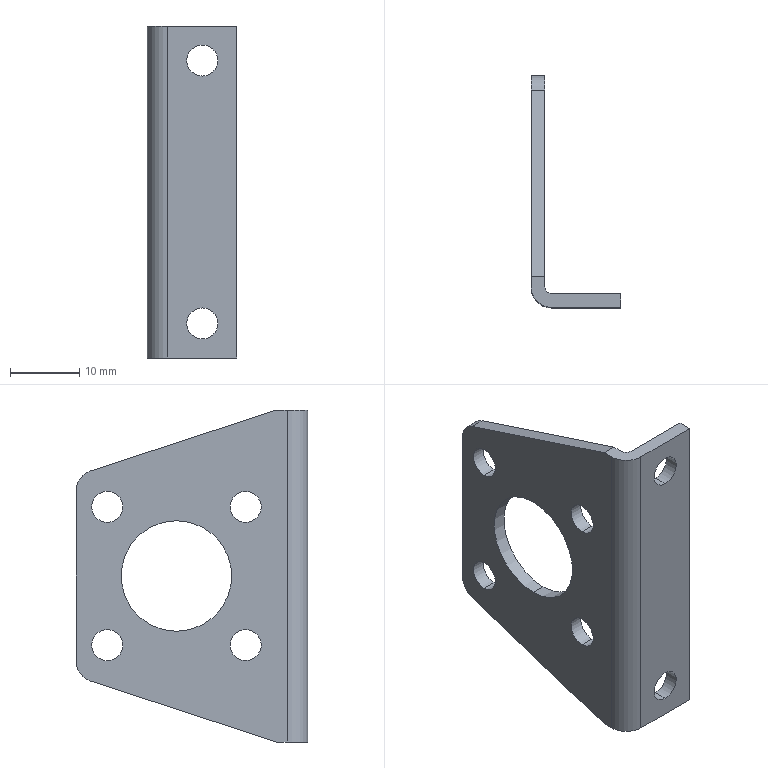Part | STEP file | _F-ACQ16LB | 1 solid | 28 faces | box 13 x 33.5 x 48 mm | volume 3042 mm3 | cylinder 18 | plane 10 | commonest cylinder face diameters 4.5 x12 6 x3 16 x2 2 x1
STEP:
#1=CARTESIAN_POINT('',(0.,19.,8.));
#2=VERTEX_POINT('',#1);
#3=CARTESIAN_POINT('',(0.,19.,-8.));
#4=VERTEX_POINT('',#3);
#5=CARTESIAN_POINT('',(0.,19.,0.));
#6=DIRECTION('',(1.,0.,0.));
#7=DIRECTION('',(0.,0.,-1.));
#8=AXIS2_PLACEMENT_3D('',#5,#6,#7);
#9=CIRCLE('',#8,8.);
#10=EDGE_CURVE('',#2,#4,#9,.T.);
#11=ORIENTED_EDGE('',*,*,#10,.F.);
#12=CARTESIAN_POINT('',(2.,19.,8.));
#13=VERTEX_POINT('',#12);
#14=CARTESIAN_POINT('',(22.,19.,8.));
#15=DIRECTION('',(1.,0.,0.));
#16=VECTOR('',#15,1000.);
#17=LINE('',#14,#16);
#18=EDGE_CURVE('',#2,#13,#17,.T.);
#19=ORIENTED_EDGE('',*,*,#18,.T.);
#20=CARTESIAN_POINT('',(2.,19.,-8.));
#21=VERTEX_POINT('',#20);
#22=CARTESIAN_POINT('',(2.,19.,0.));
#23=DIRECTION('',(1.,0.,0.));
#24=DIRECTION('',(0.,0.,-1.));
#25=AXIS2_PLACEMENT_3D('',#22,#23,#24);
#26=CIRCLE('',#25,8.);
#27=EDGE_CURVE('',#13,#21,#26,.T.);
#28=ORIENTED_EDGE('',*,*,#27,.T.);
#29=CARTESIAN_POINT('',(22.,19.,-8.));
#30=DIRECTION('',(1.,0.,0.));
#31=VECTOR('',#30,1000.);
#32=LINE('',#29,#31);
#33=EDGE_CURVE('',#4,#21,#32,.T.);
#34=ORIENTED_EDGE('',*,*,#33,.F.);
#35=EDGE_LOOP('',(#11,#19,#28,#34));
#36=FACE_OUTER_BOUND('',#35,.T.);
#37=CARTESIAN_POINT('',(22.,19.,0.));
#38=DIRECTION('',(1.,0.,0.));
#39=DIRECTION('',(0.,0.,-1.));
#40=AXIS2_PLACEMENT_3D('',#37,#38,#39);
#41=CYLINDRICAL_SURFACE('',#40,8.);
#42=ADVANCED_FACE('',(#36),#41,.F.);
#43=CARTESIAN_POINT('',(0.,9.,12.25));
#44=VERTEX_POINT('',#43);
#45=CARTESIAN_POINT('',(0.,9.,7.75));
#46=VERTEX_POINT('',#45);
#47=CARTESIAN_POINT('',(0.,9.,10.));
#48=DIRECTION('',(1.,0.,0.));
#49=DIRECTION('',(0.,0.,-1.));
#50=AXIS2_PLACEMENT_3D('',#47,#48,#49);
#51=CIRCLE('',#50,2.25);
#52=EDGE_CURVE('',#44,#46,#51,.T.);
#53=ORIENTED_EDGE('',*,*,#52,.F.);
#54=CARTESIAN_POINT('',(2.,9.,12.25));
#55=VERTEX_POINT('',#54);
#56=CARTESIAN_POINT('',(22.,9.,12.25));
#57=DIRECTION('',(1.,0.,0.));
#58=VECTOR('',#57,1000.);
#59=LINE('',#56,#58);
#60=EDGE_CURVE('',#44,#55,#59,.T.);
#61=ORIENTED_EDGE('',*,*,#60,.T.);
#62=CARTESIAN_POINT('',(2.,9.,7.75));
#63=VERTEX_POINT('',#62);
#64=CARTESIAN_POINT('',(2.,9.,10.));
#65=DIRECTION('',(1.,0.,0.));
#66=DIRECTION('',(0.,0.,-1.));
#67=AXIS2_PLACEMENT_3D('',#64,#65,#66);
#68=CIRCLE('',#67,2.25);
#69=EDGE_CURVE('',#55,#63,#68,.T.);
#70=ORIENTED_EDGE('',*,*,#69,.T.);
#71=CARTESIAN_POINT('',(22.,9.,7.75));
#72=DIRECTION('',(1.,0.,0.));
#73=VECTOR('',#72,1000.);
#74=LINE('',#71,#73);
#75=EDGE_CURVE('',#46,#63,#74,.T.);
#76=ORIENTED_EDGE('',*,*,#75,.F.);
#77=EDGE_LOOP('',(#53,#61,#70,#76));
#78=FACE_OUTER_BOUND('',#77,.T.);
#79=CARTESIAN_POINT('',(22.,9.,10.));
#80=DIRECTION('',(1.,0.,0.));
#81=DIRECTION('',(0.,0.,-1.));
#82=AXIS2_PLACEMENT_3D('',#79,#80,#81);
#83=CYLINDRICAL_SURFACE('',#82,2.25);
#84=ADVANCED_FACE('',(#78),#83,.F.);
#85=CARTESIAN_POINT('',(0.,29.,12.25));
#86=VERTEX_POINT('',#85);
#87=CARTESIAN_POINT('',(0.,29.,7.75));
#88=VERTEX_POINT('',#87);
#89=CARTESIAN_POINT('',(0.,29.,10.));
#90=DIRECTION('',(1.,0.,0.));
#91=DIRECTION('',(0.,0.,-1.));
#92=AXIS2_PLACEMENT_3D('',#89,#90,#91);
#93=CIRCLE('',#92,2.25);
#94=EDGE_CURVE('',#86,#88,#93,.T.);
#95=ORIENTED_EDGE('',*,*,#94,.F.);
#96=CARTESIAN_POINT('',(2.,29.,12.25));
#97=VERTEX_POINT('',#96);
#98=CARTESIAN_POINT('',(22.,29.,12.25));
#99=DIRECTION('',(1.,0.,0.));
#100=VECTOR('',#99,1000.);
#101=LINE('',#98,#100);
#102=EDGE_CURVE('',#86,#97,#101,.T.);
#103=ORIENTED_EDGE('',*,*,#102,.T.);
#104=CARTESIAN_POINT('',(2.,29.,7.75));
#105=VERTEX_POINT('',#104);
#106=CARTESIAN_POINT('',(2.,29.,10.));
#107=DIRECTION('',(1.,0.,0.));
#108=DIRECTION('',(0.,0.,-1.));
#109=AXIS2_PLACEMENT_3D('',#106,#107,#108);
#110=CIRCLE('',#109,2.25);
#111=EDGE_CURVE('',#97,#105,#110,.T.);
#112=ORIENTED_EDGE('',*,*,#111,.T.);
#113=CARTESIAN_POINT('',(22.,29.,7.75));
#114=DIRECTION('',(1.,0.,0.));
#115=VECTOR('',#114,1000.);
#116=LINE('',#113,#115);
#117=EDGE_CURVE('',#88,#105,#116,.T.);
#118=ORIENTED_EDGE('',*,*,#117,.F.);
#119=EDGE_LOOP('',(#95,#103,#112,#118));
#120=FACE_OUTER_BOUND('',#119,.T.);
#121=CARTESIAN_POINT('',(22.,29.,10.));
#122=DIRECTION('',(1.,0.,0.));
#123=DIRECTION('',(0.,0.,-1.));
#124=AXIS2_PLACEMENT_3D('',#121,#122,#123);
#125=CYLINDRICAL_SURFACE('',#124,2.25);
#126=ADVANCED_FACE('',(#120),#125,.F.);
#127=CARTESIAN_POINT('',(0.,29.,-7.75));
#128=VERTEX_POINT('',#127);
#129=CARTESIAN_POINT('',(0.,29.,-12.25));
#130=VERTEX_POINT('',#129);
#131=CARTESIAN_POINT('',(0.,29.,-10.));
#132=DIRECTION('',(1.,0.,0.));
#133=DIRECTION('',(0.,0.,-1.));
#134=AXIS2_PLACEMENT_3D('',#131,#132,#133);
#135=CIRCLE('',#134,2.25);
#136=EDGE_CURVE('',#128,#130,#135,.T.);
#137=ORIENTED_EDGE('',*,*,#136,.F.);
#138=CARTESIAN_POINT('',(2.,29.,-7.75));
#139=VERTEX_POINT('',#138);
#140=CARTESIAN_POINT('',(22.,29.,-7.75));
#141=DIRECTION('',(1.,0.,0.));
#142=VECTOR('',#141,1000.);
#143=LINE('',#140,#142);
#144=EDGE_CURVE('',#128,#139,#143,.T.);
#145=ORIENTED_EDGE('',*,*,#144,.T.);
#146=CARTESIAN_POINT('',(2.,29.,-12.25));
#147=VERTEX_POINT('',#146);
#148=CARTESIAN_POINT('',(2.,29.,-10.));
#149=DIRECTION('',(1.,0.,0.));
#150=DIRECTION('',(0.,0.,-1.));
#151=AXIS2_PLACEMENT_3D('',#148,#149,#150);
#152=CIRCLE('',#151,2.25);
#153=EDGE_CURVE('',#139,#147,#152,.T.);
#154=ORIENTED_EDGE('',*,*,#153,.T.);
#155=CARTESIAN_POINT('',(22.,29.,-12.25));
#156=DIRECTION('',(1.,0.,0.));
#157=VECTOR('',#156,1000.);
#158=LINE('',#155,#157);
#159=EDGE_CURVE('',#130,#147,#158,.T.);
#160=ORIENTED_EDGE('',*,*,#159,.F.);
#161=EDGE_LOOP('',(#137,#145,#154,#160));
#162=FACE_OUTER_BOUND('',#161,.T.);
#163=CARTESIAN_POINT('',(22.,29.,-10.));
#164=DIRECTION('',(1.,0.,0.));
#165=DIRECTION('',(0.,0.,-1.));
#166=AXIS2_PLACEMENT_3D('',#163,#164,#165);
#167=CYLINDRICAL_SURFACE('',#166,2.25);
#168=ADVANCED_FACE('',(#162),#167,.F.);
#169=CARTESIAN_POINT('',(0.,9.,-7.75));
#170=VERTEX_POINT('',#169);
#171=CARTESIAN_POINT('',(0.,9.,-12.25));
#172=VERTEX_POINT('',#171);
#173=CARTESIAN_POINT('',(0.,9.,-10.));
#174=DIRECTION('',(1.,0.,0.));
#175=DIRECTION('',(0.,0.,-1.));
#176=AXIS2_PLACEMENT_3D('',#173,#174,#175);
#177=CIRCLE('',#176,2.25);
#178=EDGE_CURVE('',#170,#172,#177,.T.);
#179=ORIENTED_EDGE('',*,*,#178,.F.);
#180=CARTESIAN_POINT('',(2.,9.,-7.75));
#181=VERTEX_POINT('',#180);
#182=CARTESIAN_POINT('',(22.,9.,-7.75));
#183=DIRECTION('',(1.,0.,0.));
#184=VECTOR('',#183,1000.);
#185=LINE('',#182,#184);
#186=EDGE_CURVE('',#170,#181,#185,.T.);
#187=ORIENTED_EDGE('',*,*,#186,.T.);
#188=CARTESIAN_POINT('',(2.,9.,-12.25));
#189=VERTEX_POINT('',#188);
#190=CARTESIAN_POINT('',(2.,9.,-10.));
#191=DIRECTION('',(1.,0.,0.));
#192=DIRECTION('',(0.,0.,-1.));
#193=AXIS2_PLACEMENT_3D('',#190,#191,#192);
#194=CIRCLE('',#193,2.25);
#195=EDGE_CURVE('',#181,#189,#194,.T.);
#196=ORIENTED_EDGE('',*,*,#195,.T.);
#197=CARTESIAN_POINT('',(22.,9.,-12.25));
#198=DIRECTION('',(1.,0.,0.));
#199=VECTOR('',#198,1000.);
#200=LINE('',#197,#199);
#201=EDGE_CURVE('',#172,#189,#200,.T.);
#202=ORIENTED_EDGE('',*,*,#201,.F.);
#203=EDGE_LOOP('',(#179,#187,#196,#202));
#204=FACE_OUTER_BOUND('',#203,.T.);
#205=CARTESIAN_POINT('',(22.,9.,-10.));
#206=DIRECTION('',(1.,0.,0.));
#207=DIRECTION('',(0.,0.,-1.));
#208=AXIS2_PLACEMENT_3D('',#205,#206,#207);
#209=CYLINDRICAL_SURFACE('',#208,2.25);
#210=ADVANCED_FACE('',(#204),#209,.F.);
#211=CARTESIAN_POINT('',(8.,0.,-16.75));
#212=VERTEX_POINT('',#211);
#213=CARTESIAN_POINT('',(8.,0.,-21.25));
#214=VERTEX_POINT('',#213);
#215=CARTESIAN_POINT('',(8.,0.,-19.));
#216=DIRECTION('',(0.,-1.,0.));
#217=DIRECTION('',(0.,0.,1.));
#218=AXIS2_PLACEMENT_3D('',#215,#216,#217);
#219=CIRCLE('',#218,2.25);
#220=EDGE_CURVE('',#212,#214,#219,.T.);
#221=ORIENTED_EDGE('',*,*,#220,.T.);
#222=CARTESIAN_POINT('',(8.,2.,-21.25));
#223=VERTEX_POINT('',#222);
#224=CARTESIAN_POINT('',(8.,24.,-21.25));
#225=DIRECTION('',(0.,1.,0.));
#226=VECTOR('',#225,1000.);
#227=LINE('',#224,#226);
#228=EDGE_CURVE('',#214,#223,#227,.T.);
#229=ORIENTED_EDGE('',*,*,#228,.T.);
#230=CARTESIAN_POINT('',(8.,2.,-16.75));
#231=VERTEX_POINT('',#230);
#232=CARTESIAN_POINT('',(8.,2.,-19.));
#233=DIRECTION('',(0.,1.,0.));
#234=DIRECTION('',(0.,0.,1.));
#235=AXIS2_PLACEMENT_3D('',#232,#233,#234);
#236=CIRCLE('',#235,2.25);
#237=EDGE_CURVE('',#223,#231,#236,.T.);
#238=ORIENTED_EDGE('',*,*,#237,.T.);
#239=CARTESIAN_POINT('',(8.,24.,-16.75));
#240=DIRECTION('',(0.,1.,0.));
#241=VECTOR('',#240,1000.);
#242=LINE('',#239,#241);
#243=EDGE_CURVE('',#212,#231,#242,.T.);
#244=ORIENTED_EDGE('',*,*,#243,.F.);
#245=EDGE_LOOP('',(#221,#229,#238,#244));
#246=FACE_OUTER_BOUND('',#245,.T.);
#247=CARTESIAN_POINT('',(8.,24.,-19.));
#248=DIRECTION('',(0.,1.,0.));
#249=DIRECTION('',(0.,0.,1.));
#250=AXIS2_PLACEMENT_3D('',#247,#248,#249);
#251=CYLINDRICAL_SURFACE('',#250,2.25);
#252=ADVANCED_FACE('',(#246),#251,.F.);
#253=CARTESIAN_POINT('',(8.,0.,21.25));
#254=VERTEX_POINT('',#253);
#255=CARTESIAN_POINT('',(8.,0.,16.75));
#256=VERTEX_POINT('',#255);
#257=CARTESIAN_POINT('',(8.,0.,19.));
#258=DIRECTION('',(0.,-1.,0.));
#259=DIRECTION('',(0.,0.,1.));
#260=AXIS2_PLACEMENT_3D('',#257,#258,#259);
#261=CIRCLE('',#260,2.25);
#262=EDGE_CURVE('',#254,#256,#261,.T.);
#263=ORIENTED_EDGE('',*,*,#262,.T.);
#264=CARTESIAN_POINT('',(8.,2.,16.75));
#265=VERTEX_POINT('',#264);
#266=CARTESIAN_POINT('',(8.,24.,16.75));
#267=DIRECTION('',(0.,1.,0.));
#268=VECTOR('',#267,1000.);
#269=LINE('',#266,#268);
#270=EDGE_CURVE('',#256,#265,#269,.T.);
#271=ORIENTED_EDGE('',*,*,#270,.T.);
#272=CARTESIAN_POINT('',(8.,2.,21.25));
#273=VERTEX_POINT('',#272);
#274=CARTESIAN_POINT('',(8.,2.,19.));
#275=DIRECTION('',(0.,1.,0.));
#276=DIRECTION('',(0.,0.,1.));
#277=AXIS2_PLACEMENT_3D('',#274,#275,#276);
#278=CIRCLE('',#277,2.25);
#279=EDGE_CURVE('',#265,#273,#278,.T.);
#280=ORIENTED_EDGE('',*,*,#279,.T.);
#281=CARTESIAN_POINT('',(8.,24.,21.25));
#282=DIRECTION('',(0.,1.,0.));
#283=VECTOR('',#282,1000.);
#284=LINE('',#281,#283);
#285=EDGE_CURVE('',#254,#273,#284,.T.);
#286=ORIENTED_EDGE('',*,*,#285,.F.);
#287=EDGE_LOOP('',(#263,#271,#280,#286));
#288=FACE_OUTER_BOUND('',#287,.T.);
#289=CARTESIAN_POINT('',(8.,24.,19.));
#290=DIRECTION('',(0.,1.,0.));
#291=DIRECTION('',(0.,0.,1.));
#292=AXIS2_PLACEMENT_3D('',#289,#290,#291);
#293=CYLINDRICAL_SURFACE('',#292,2.25);
#294=ADVANCED_FACE('',(#288),#293,.F.);
#295=CARTESIAN_POINT('',(2.,4.5,24.));
#296=VERTEX_POINT('',#295);
#297=CARTESIAN_POINT('',(2.,31.434,15.181));
#298=VERTEX_POINT('',#297);
#299=CARTESIAN_POINT('',(2.,4.5,24.));
#300=DIRECTION('',(0.,0.9504,-0.3112));
#301=VECTOR('',#300,1000.);
#302=LINE('',#299,#301);
#303=EDGE_CURVE('',#296,#298,#302,.T.);
#304=ORIENTED_EDGE('',*,*,#303,.F.);
#305=CARTESIAN_POINT('',(2.,3.,24.));
#306=VERTEX_POINT('',#305);
#307=CARTESIAN_POINT('',(2.,3.,24.));
#308=DIRECTION('',(0.,1.,0.));
#309=VECTOR('',#308,1000.);
#310=LINE('',#307,#309);
#311=EDGE_CURVE('',#306,#296,#310,.T.);
#312=ORIENTED_EDGE('',*,*,#311,.F.);
#313=CARTESIAN_POINT('',(2.,3.,-24.));
#314=VERTEX_POINT('',#313);
#315=CARTESIAN_POINT('',(2.,3.,24.));
#316=DIRECTION('',(0.,0.,1.));
#317=VECTOR('',#316,1000.);
#318=LINE('',#315,#317);
#319=EDGE_CURVE('',#314,#306,#318,.T.);
#320=ORIENTED_EDGE('',*,*,#319,.F.);
#321=CARTESIAN_POINT('',(2.,4.5,-24.));
#322=VERTEX_POINT('',#321);
#323=CARTESIAN_POINT('',(2.,3.,-24.));
#324=DIRECTION('',(0.,1.,0.));
#325=VECTOR('',#324,1000.);
#326=LINE('',#323,#325);
#327=EDGE_CURVE('',#314,#322,#326,.T.);
#328=ORIENTED_EDGE('',*,*,#327,.T.);
#329=CARTESIAN_POINT('',(2.,31.434,-15.181));
#330=VERTEX_POINT('',#329);
#331=CARTESIAN_POINT('',(2.,31.434,-15.181));
#332=DIRECTION('',(0.,-0.9504,-0.3112));
#333=VECTOR('',#332,1000.);
#334=LINE('',#331,#333);
#335=EDGE_CURVE('',#330,#322,#334,.T.);
#336=ORIENTED_EDGE('',*,*,#335,.F.);
#337=CARTESIAN_POINT('',(2.,33.5,-12.33));
#338=VERTEX_POINT('',#337);
#339=CARTESIAN_POINT('',(2.,30.5,-12.33));
#340=DIRECTION('',(-1.,0.,0.));
#341=DIRECTION('',(0.,0.,-1.));
#342=AXIS2_PLACEMENT_3D('',#339,#340,#341);
#343=CIRCLE('',#342,3.);
#344=EDGE_CURVE('',#338,#330,#343,.T.);
#345=ORIENTED_EDGE('',*,*,#344,.F.);
#346=CARTESIAN_POINT('',(2.,33.5,12.33));
#347=VERTEX_POINT('',#346);
#348=CARTESIAN_POINT('',(2.,33.5,24.));
#349=DIRECTION('',(0.,0.,-1.));
#350=VECTOR('',#349,1000.);
#351=LINE('',#348,#350);
#352=EDGE_CURVE('',#347,#338,#351,.T.);
#353=ORIENTED_EDGE('',*,*,#352,.F.);
#354=CARTESIAN_POINT('',(2.,30.5,12.33));
#355=DIRECTION('',(-1.,0.,0.));
#356=DIRECTION('',(0.,0.,-1.));
#357=AXIS2_PLACEMENT_3D('',#354,#355,#356);
#358=CIRCLE('',#357,3.);
#359=EDGE_CURVE('',#298,#347,#358,.T.);
#360=ORIENTED_EDGE('',*,*,#359,.F.);
#361=EDGE_LOOP('',(#304,#312,#320,#328,#336,#345,#353,#360));
#362=FACE_OUTER_BOUND('',#361,.T.);
#363=CARTESIAN_POINT('',(2.,19.,0.));
#364=DIRECTION('',(1.,0.,0.));
#365=DIRECTION('',(0.,0.,-1.));
#366=AXIS2_PLACEMENT_3D('',#363,#364,#365);
#367=CIRCLE('',#366,8.);
#368=EDGE_CURVE('',#21,#13,#367,.T.);
#369=ORIENTED_EDGE('',*,*,#368,.F.);
#370=ORIENTED_EDGE('',*,*,#27,.F.);
#371=EDGE_LOOP('',(#369,#370));
#372=FACE_BOUND('',#371,.T.);
#373=CARTESIAN_POINT('',(2.,9.,10.));
#374=DIRECTION('',(1.,0.,0.));
#375=DIRECTION('',(0.,0.,-1.));
#376=AXIS2_PLACEMENT_3D('',#373,#374,#375);
#377=CIRCLE('',#376,2.25);
#378=EDGE_CURVE('',#63,#55,#377,.T.);
#379=ORIENTED_EDGE('',*,*,#378,.F.);
#380=ORIENTED_EDGE('',*,*,#69,.F.);
#381=EDGE_LOOP('',(#379,#380));
#382=FACE_BOUND('',#381,.T.);
#383=CARTESIAN_POINT('',(2.,29.,10.));
#384=DIRECTION('',(1.,0.,0.));
#385=DIRECTION('',(0.,0.,-1.));
#386=AXIS2_PLACEMENT_3D('',#383,#384,#385);
#387=CIRCLE('',#386,2.25);
#388=EDGE_CURVE('',#105,#97,#387,.T.);
#389=ORIENTED_EDGE('',*,*,#388,.F.);
#390=ORIENTED_EDGE('',*,*,#111,.F.);
#391=EDGE_LOOP('',(#389,#390));
#392=FACE_BOUND('',#391,.T.);
#393=CARTESIAN_POINT('',(2.,29.,-10.));
#394=DIRECTION('',(1.,0.,0.));
#395=DIRECTION('',(0.,0.,-1.));
#396=AXIS2_PLACEMENT_3D('',#393,#394,#395);
#397=CIRCLE('',#396,2.25);
#398=EDGE_CURVE('',#147,#139,#397,.T.);
#399=ORIENTED_EDGE('',*,*,#398,.F.);
#400=ORIENTED_EDGE('',*,*,#153,.F.);
#401=EDGE_LOOP('',(#399,#400));
#402=FACE_BOUND('',#401,.T.);
#403=CARTESIAN_POINT('',(2.,9.,-10.));
#404=DIRECTION('',(1.,0.,0.));
#405=DIRECTION('',(0.,0.,-1.));
#406=AXIS2_PLACEMENT_3D('',#403,#404,#405);
#407=CIRCLE('',#406,2.25);
#408=EDGE_CURVE('',#189,#181,#407,.T.);
#409=ORIENTED_EDGE('',*,*,#408,.F.);
#410=ORIENTED_EDGE('',*,*,#195,.F.);
#411=EDGE_LOOP('',(#409,#410));
#412=FACE_BOUND('',#411,.T.);
#413=CARTESIAN_POINT('',(2.,3.,24.));
#414=DIRECTION('',(-1.,0.,0.));
#415=DIRECTION('',(0.,0.,1.));
#416=AXIS2_PLACEMENT_3D('',#413,#414,#415);
#417=PLANE('',#416);
#418=ADVANCED_FACE('',(#362,#372,#382,#392,#402,#412),#417,.F.);
#419=CARTESIAN_POINT('',(0.,33.5,12.33));
#420=VERTEX_POINT('',#419);
#421=CARTESIAN_POINT('',(22.,33.5,12.33));
#422=DIRECTION('',(-1.,0.,0.));
#423=VECTOR('',#422,1000.);
#424=LINE('',#421,#423);
#425=EDGE_CURVE('',#347,#420,#424,.T.);
#426=ORIENTED_EDGE('',*,*,#425,.T.);
#427=CARTESIAN_POINT('',(0.,31.434,15.181));
#428=VERTEX_POINT('',#427);
#429=CARTESIAN_POINT('',(0.,30.5,12.33));
#430=DIRECTION('',(1.,0.,0.));
#431=DIRECTION('',(0.,0.,-1.));
#432=AXIS2_PLACEMENT_3D('',#429,#430,#431);
#433=CIRCLE('',#432,3.);
#434=EDGE_CURVE('',#420,#428,#433,.T.);
#435=ORIENTED_EDGE('',*,*,#434,.T.);
#436=CARTESIAN_POINT('',(22.,31.434,15.181));
#437=DIRECTION('',(1.,0.,0.));
#438=VECTOR('',#437,1000.);
#439=LINE('',#436,#438);
#440=EDGE_CURVE('',#428,#298,#439,.T.);
#441=ORIENTED_EDGE('',*,*,#440,.T.);
#442=ORIENTED_EDGE('',*,*,#359,.T.);
#443=EDGE_LOOP('',(#426,#435,#441,#442));
#444=FACE_OUTER_BOUND('',#443,.T.);
#445=CARTESIAN_POINT('',(22.,30.5,12.33));
#446=DIRECTION('',(1.,0.,0.));
#447=DIRECTION('',(0.,0.,-1.));
#448=AXIS2_PLACEMENT_3D('',#445,#446,#447);
#449=CYLINDRICAL_SURFACE('',#448,3.);
#450=ADVANCED_FACE('',(#444),#449,.T.);
#451=ORIENTED_EDGE('',*,*,#303,.T.);
#452=ORIENTED_EDGE('',*,*,#440,.F.);
#453=CARTESIAN_POINT('',(0.,4.5,24.));
#454=VERTEX_POINT('',#453);
#455=CARTESIAN_POINT('',(0.,31.434,15.181));
#456=DIRECTION('',(0.,0.9504,-0.3112));
#457=VECTOR('',#456,1000.);
#458=LINE('',#455,#457);
#459=EDGE_CURVE('',#454,#428,#458,.T.);
#460=ORIENTED_EDGE('',*,*,#459,.F.);
#461=CARTESIAN_POINT('',(22.,4.5,24.));
#462=DIRECTION('',(-1.,0.,0.));
#463=VECTOR('',#462,1000.);
#464=LINE('',#461,#463);
#465=EDGE_CURVE('',#296,#454,#464,.T.);
#466=ORIENTED_EDGE('',*,*,#465,.F.);
#467=EDGE_LOOP('',(#451,#452,#460,#466));
#468=FACE_OUTER_BOUND('',#467,.T.);
#469=CARTESIAN_POINT('',(22.,31.434,15.181));
#470=DIRECTION('',(0.,-0.3112,-0.9504));
#471=DIRECTION('',(0.,0.9504,-0.3112));
#472=AXIS2_PLACEMENT_3D('',#469,#470,#471);
#473=PLANE('',#472);
#474=ADVANCED_FACE('',(#468),#473,.F.);
#475=ORIENTED_EDGE('',*,*,#319,.T.);
#476=CARTESIAN_POINT('',(3.,2.,24.));
#477=VERTEX_POINT('',#476);
#478=CARTESIAN_POINT('',(3.,3.,24.));
#479=DIRECTION('',(0.,0.,-1.));
#480=DIRECTION('',(1.,0.,0.));
#481=AXIS2_PLACEMENT_3D('',#478,#479,#480);
#482=CIRCLE('',#481,1.);
#483=EDGE_CURVE('',#477,#306,#482,.T.);
#484=ORIENTED_EDGE('',*,*,#483,.F.);
#485=CARTESIAN_POINT('',(3.,2.,-24.));
#486=VERTEX_POINT('',#485);
#487=CARTESIAN_POINT('',(3.,2.,24.));
#488=DIRECTION('',(0.,0.,1.));
#489=VECTOR('',#488,1000.);
#490=LINE('',#487,#489);
#491=EDGE_CURVE('',#486,#477,#490,.T.);
#492=ORIENTED_EDGE('',*,*,#491,.F.);
#493=CARTESIAN_POINT('',(3.,3.,-24.));
#494=DIRECTION('',(0.,0.,-1.));
#495=DIRECTION('',(1.,0.,0.));
#496=AXIS2_PLACEMENT_3D('',#493,#494,#495);
#497=CIRCLE('',#496,1.);
#498=EDGE_CURVE('',#486,#314,#497,.T.);
#499=ORIENTED_EDGE('',*,*,#498,.T.);
#500=EDGE_LOOP('',(#475,#484,#492,#499));
#501=FACE_OUTER_BOUND('',#500,.T.);
#502=CARTESIAN_POINT('',(3.,3.,24.));
#503=DIRECTION('',(0.,0.,1.));
#504=DIRECTION('',(1.,0.,0.));
#505=AXIS2_PLACEMENT_3D('',#502,#503,#504);
#506=CYLINDRICAL_SURFACE('',#505,1.);
#507=ADVANCED_FACE('',(#501),#506,.F.);
#508=ORIENTED_EDGE('',*,*,#335,.T.);
#509=CARTESIAN_POINT('',(0.,4.5,-24.));
#510=VERTEX_POINT('',#509);
#511=CARTESIAN_POINT('',(22.,4.5,-24.));
#512=DIRECTION('',(1.,0.,0.));
#513=VECTOR('',#512,1000.);
#514=LINE('',#511,#513);
#515=EDGE_CURVE('',#510,#322,#514,.T.);
#516=ORIENTED_EDGE('',*,*,#515,.F.);
#517=CARTESIAN_POINT('',(0.,31.434,-15.181));
#518=VERTEX_POINT('',#517);
#519=CARTESIAN_POINT('',(0.,4.5,-24.));
#520=DIRECTION('',(0.,-0.9504,-0.3112));
#521=VECTOR('',#520,1000.);
#522=LINE('',#519,#521);
#523=EDGE_CURVE('',#518,#510,#522,.T.);
#524=ORIENTED_EDGE('',*,*,#523,.F.);
#525=CARTESIAN_POINT('',(22.,31.434,-15.181));
#526=DIRECTION('',(-1.,0.,0.));
#527=VECTOR('',#526,1000.);
#528=LINE('',#525,#527);
#529=EDGE_CURVE('',#330,#518,#528,.T.);
#530=ORIENTED_EDGE('',*,*,#529,.F.);
#531=EDGE_LOOP('',(#508,#516,#524,#530));
#532=FACE_OUTER_BOUND('',#531,.T.);
#533=CARTESIAN_POINT('',(22.,4.5,-24.));
#534=DIRECTION('',(0.,-0.3112,0.9504));
#535=DIRECTION('',(0.,-0.9504,-0.3112));
#536=AXIS2_PLACEMENT_3D('',#533,#534,#535);
#537=PLANE('',#536);
#538=ADVANCED_FACE('',(#532),#537,.F.);
#539=ORIENTED_EDGE('',*,*,#529,.T.);
#540=CARTESIAN_POINT('',(0.,33.5,-12.33));
#541=VERTEX_POINT('',#540);
#542=CARTESIAN_POINT('',(0.,30.5,-12.33));
#543=DIRECTION('',(1.,0.,0.));
#544=DIRECTION('',(0.,0.,-1.));
#545=AXIS2_PLACEMENT_3D('',#542,#543,#544);
#546=CIRCLE('',#545,3.);
#547=EDGE_CURVE('',#518,#541,#546,.T.);
#548=ORIENTED_EDGE('',*,*,#547,.T.);
#549=CARTESIAN_POINT('',(22.,33.5,-12.33));
#550=DIRECTION('',(1.,0.,0.));
#551=VECTOR('',#550,1000.);
#552=LINE('',#549,#551);
#553=EDGE_CURVE('',#541,#338,#552,.T.);
#554=ORIENTED_EDGE('',*,*,#553,.T.);
#555=ORIENTED_EDGE('',*,*,#344,.T.);
#556=EDGE_LOOP('',(#539,#548,#554,#555));
#557=FACE_OUTER_BOUND('',#556,.T.);
#558=CARTESIAN_POINT('',(22.,30.5,-12.33));
#559=DIRECTION('',(1.,0.,0.));
#560=DIRECTION('',(0.,0.,-1.));
#561=AXIS2_PLACEMENT_3D('',#558,#559,#560);
#562=CYLINDRICAL_SURFACE('',#561,3.);
#563=ADVANCED_FACE('',(#557),#562,.T.);
#564=ORIENTED_EDGE('',*,*,#425,.F.);
#565=ORIENTED_EDGE('',*,*,#352,.T.);
#566=ORIENTED_EDGE('',*,*,#553,.F.);
#567=CARTESIAN_POINT('',(0.,33.5,24.));
#568=DIRECTION('',(0.,0.,-1.));
#569=VECTOR('',#568,1000.);
#570=LINE('',#567,#569);
#571=EDGE_CURVE('',#420,#541,#570,.T.);
#572=ORIENTED_EDGE('',*,*,#571,.F.);
#573=EDGE_LOOP('',(#564,#565,#566,#572));
#574=FACE_OUTER_BOUND('',#573,.T.);
#575=CARTESIAN_POINT('',(2.,33.5,24.));
#576=DIRECTION('',(0.,-1.,0.));
#577=DIRECTION('',(0.,0.,-1.));
#578=AXIS2_PLACEMENT_3D('',#575,#576,#577);
#579=PLANE('',#578);
#580=ADVANCED_FACE('',(#574),#579,.F.);
#581=ORIENTED_EDGE('',*,*,#18,.F.);
#582=CARTESIAN_POINT('',(0.,19.,0.));
#583=DIRECTION('',(1.,0.,0.));
#584=DIRECTION('',(0.,0.,-1.));
#585=AXIS2_PLACEMENT_3D('',#582,#583,#584);
#586=CIRCLE('',#585,8.);
#587=EDGE_CURVE('',#4,#2,#586,.T.);
#588=ORIENTED_EDGE('',*,*,#587,.F.);
#589=ORIENTED_EDGE('',*,*,#33,.T.);
#590=ORIENTED_EDGE('',*,*,#368,.T.);
#591=EDGE_LOOP('',(#581,#588,#589,#590));
#592=FACE_OUTER_BOUND('',#591,.T.);
#593=CARTESIAN_POINT('',(22.,19.,0.));
#594=DIRECTION('',(1.,0.,0.));
#595=DIRECTION('',(0.,0.,-1.));
#596=AXIS2_PLACEMENT_3D('',#593,#594,#595);
#597=CYLINDRICAL_SURFACE('',#596,8.);
#598=ADVANCED_FACE('',(#592),#597,.F.);
#599=ORIENTED_EDGE('',*,*,#60,.F.);
#600=CARTESIAN_POINT('',(0.,9.,10.));
#601=DIRECTION('',(1.,0.,0.));
#602=DIRECTION('',(0.,0.,-1.));
#603=AXIS2_PLACEMENT_3D('',#600,#601,#602);
#604=CIRCLE('',#603,2.25);
#605=EDGE_CURVE('',#46,#44,#604,.T.);
#606=ORIENTED_EDGE('',*,*,#605,.F.);
#607=ORIENTED_EDGE('',*,*,#75,.T.);
#608=ORIENTED_EDGE('',*,*,#378,.T.);
#609=EDGE_LOOP('',(#599,#606,#607,#608));
#610=FACE_OUTER_BOUND('',#609,.T.);
#611=CARTESIAN_POINT('',(22.,9.,10.));
#612=DIRECTION('',(1.,0.,0.));
#613=DIRECTION('',(0.,0.,-1.));
#614=AXIS2_PLACEMENT_3D('',#611,#612,#613);
#615=CYLINDRICAL_SURFACE('',#614,2.25);
#616=ADVANCED_FACE('',(#610),#615,.F.);
#617=ORIENTED_EDGE('',*,*,#102,.F.);
#618=CARTESIAN_POINT('',(0.,29.,10.));
#619=DIRECTION('',(1.,0.,0.));
#620=DIRECTION('',(0.,0.,-1.));
#621=AXIS2_PLACEMENT_3D('',#618,#619,#620);
#622=CIRCLE('',#621,2.25);
#623=EDGE_CURVE('',#88,#86,#622,.T.);
#624=ORIENTED_EDGE('',*,*,#623,.F.);
#625=ORIENTED_EDGE('',*,*,#117,.T.);
#626=ORIENTED_EDGE('',*,*,#388,.T.);
#627=EDGE_LOOP('',(#617,#624,#625,#626));
#628=FACE_OUTER_BOUND('',#627,.T.);
#629=CARTESIAN_POINT('',(22.,29.,10.));
#630=DIRECTION('',(1.,0.,0.));
#631=DIRECTION('',(0.,0.,-1.));
#632=AXIS2_PLACEMENT_3D('',#629,#630,#631);
#633=CYLINDRICAL_SURFACE('',#632,2.25);
#634=ADVANCED_FACE('',(#628),#633,.F.);
#635=ORIENTED_EDGE('',*,*,#144,.F.);
#636=CARTESIAN_POINT('',(0.,29.,-10.));
#637=DIRECTION('',(1.,0.,0.));
#638=DIRECTION('',(0.,0.,-1.));
#639=AXIS2_PLACEMENT_3D('',#636,#637,#638);
#640=CIRCLE('',#639,2.25);
#641=EDGE_CURVE('',#130,#128,#640,.T.);
#642=ORIENTED_EDGE('',*,*,#641,.F.);
#643=ORIENTED_EDGE('',*,*,#159,.T.);
#644=ORIENTED_EDGE('',*,*,#398,.T.);
#645=EDGE_LOOP('',(#635,#642,#643,#644));
#646=FACE_OUTER_BOUND('',#645,.T.);
#647=CARTESIAN_POINT('',(22.,29.,-10.));
#648=DIRECTION('',(1.,0.,0.));
#649=DIRECTION('',(0.,0.,-1.));
#650=AXIS2_PLACEMENT_3D('',#647,#648,#649);
#651=CYLINDRICAL_SURFACE('',#650,2.25);
#652=ADVANCED_FACE('',(#646),#651,.F.);
#653=ORIENTED_EDGE('',*,*,#186,.F.);
#654=CARTESIAN_POINT('',(0.,9.,-10.));
#655=DIRECTION('',(1.,0.,0.));
#656=DIRECTION('',(0.,0.,-1.));
#657=AXIS2_PLACEMENT_3D('',#654,#655,#656);
#658=CIRCLE('',#657,2.25);
#659=EDGE_CURVE('',#172,#170,#658,.T.);
#660=ORIENTED_EDGE('',*,*,#659,.F.);
#661=ORIENTED_EDGE('',*,*,#201,.T.);
#662=ORIENTED_EDGE('',*,*,#408,.T.);
#663=EDGE_LOOP('',(#653,#660,#661,#662));
#664=FACE_OUTER_BOUND('',#663,.T.);
#665=CARTESIAN_POINT('',(22.,9.,-10.));
#666=DIRECTION('',(1.,0.,0.));
#667=DIRECTION('',(0.,0.,-1.));
#668=AXIS2_PLACEMENT_3D('',#665,#666,#667);
#669=CYLINDRICAL_SURFACE('',#668,2.25);
#670=ADVANCED_FACE('',(#664),#669,.F.);
#671=ORIENTED_EDGE('',*,*,#459,.T.);
#672=ORIENTED_EDGE('',*,*,#434,.F.);
#673=ORIENTED_EDGE('',*,*,#571,.T.);
#674=ORIENTED_EDGE('',*,*,#547,.F.);
#675=ORIENTED_EDGE('',*,*,#523,.T.);
#676=CARTESIAN_POINT('',(0.,3.,-24.));
#677=VERTEX_POINT('',#676);
#678=CARTESIAN_POINT('',(0.,33.5,-24.));
#679=DIRECTION('',(0.,1.,0.));
#680=VECTOR('',#679,1000.);
#681=LINE('',#678,#680);
#682=EDGE_CURVE('',#677,#510,#681,.T.);
#683=ORIENTED_EDGE('',*,*,#682,.F.);
#684=CARTESIAN_POINT('',(0.,3.,24.));
#685=VERTEX_POINT('',#684);
#686=CARTESIAN_POINT('',(0.,3.,24.));
#687=DIRECTION('',(0.,0.,-1.));
#688=VECTOR('',#687,1000.);
#689=LINE('',#686,#688);
#690=EDGE_CURVE('',#685,#677,#689,.T.);
#691=ORIENTED_EDGE('',*,*,#690,.F.);
#692=CARTESIAN_POINT('',(0.,33.5,24.));
#693=DIRECTION('',(0.,-1.,0.));
#694=VECTOR('',#693,1000.);
#695=LINE('',#692,#694);
#696=EDGE_CURVE('',#454,#685,#695,.T.);
#697=ORIENTED_EDGE('',*,*,#696,.F.);
#698=EDGE_LOOP('',(#671,#672,#673,#674,#675,#683,#691,#697));
#699=FACE_OUTER_BOUND('',#698,.T.);
#700=ORIENTED_EDGE('',*,*,#587,.T.);
#701=ORIENTED_EDGE('',*,*,#10,.T.);
#702=EDGE_LOOP('',(#700,#701));
#703=FACE_BOUND('',#702,.T.);
#704=ORIENTED_EDGE('',*,*,#605,.T.);
#705=ORIENTED_EDGE('',*,*,#52,.T.);
#706=EDGE_LOOP('',(#704,#705));
#707=FACE_BOUND('',#706,.T.);
#708=ORIENTED_EDGE('',*,*,#623,.T.);
#709=ORIENTED_EDGE('',*,*,#94,.T.);
#710=EDGE_LOOP('',(#708,#709));
#711=FACE_BOUND('',#710,.T.);
#712=ORIENTED_EDGE('',*,*,#641,.T.);
#713=ORIENTED_EDGE('',*,*,#136,.T.);
#714=EDGE_LOOP('',(#712,#713));
#715=FACE_BOUND('',#714,.T.);
#716=ORIENTED_EDGE('',*,*,#659,.T.);
#717=ORIENTED_EDGE('',*,*,#178,.T.);
#718=EDGE_LOOP('',(#716,#717));
#719=FACE_BOUND('',#718,.T.);
#720=CARTESIAN_POINT('',(0.,33.5,24.));
#721=DIRECTION('',(1.,0.,0.));
#722=DIRECTION('',(0.,0.,-1.));
#723=AXIS2_PLACEMENT_3D('',#720,#721,#722);
#724=PLANE('',#723);
#725=ADVANCED_FACE('',(#699,#703,#707,#711,#715,#719),#724,.F.);
#726=ORIENTED_EDGE('',*,*,#483,.T.);
#727=ORIENTED_EDGE('',*,*,#311,.T.);
#728=ORIENTED_EDGE('',*,*,#465,.T.);
#729=ORIENTED_EDGE('',*,*,#696,.T.);
#730=CARTESIAN_POINT('',(3.,0.,24.));
#731=VERTEX_POINT('',#730);
#732=CARTESIAN_POINT('',(3.,3.,24.));
#733=DIRECTION('',(0.,0.,1.));
#734=DIRECTION('',(1.,0.,0.));
#735=AXIS2_PLACEMENT_3D('',#732,#733,#734);
#736=CIRCLE('',#735,3.);
#737=EDGE_CURVE('',#685,#731,#736,.T.);
#738=ORIENTED_EDGE('',*,*,#737,.T.);
#739=CARTESIAN_POINT('',(13.,0.,24.));
#740=VERTEX_POINT('',#739);
#741=CARTESIAN_POINT('',(3.,0.,24.));
#742=DIRECTION('',(1.,0.,0.));
#743=VECTOR('',#742,1000.);
#744=LINE('',#741,#743);
#745=EDGE_CURVE('',#731,#740,#744,.T.);
#746=ORIENTED_EDGE('',*,*,#745,.T.);
#747=CARTESIAN_POINT('',(13.,2.,24.));
#748=VERTEX_POINT('',#747);
#749=CARTESIAN_POINT('',(13.,3.,24.));
#750=DIRECTION('',(0.,1.,0.));
#751=VECTOR('',#750,1000.);
#752=LINE('',#749,#751);
#753=EDGE_CURVE('',#740,#748,#752,.T.);
#754=ORIENTED_EDGE('',*,*,#753,.T.);
#755=CARTESIAN_POINT('',(3.,2.,24.));
#756=DIRECTION('',(-1.,0.,0.));
#757=VECTOR('',#756,1000.);
#758=LINE('',#755,#757);
#759=EDGE_CURVE('',#748,#477,#758,.T.);
#760=ORIENTED_EDGE('',*,*,#759,.T.);
#761=EDGE_LOOP('',(#726,#727,#728,#729,#738,#746,#754,#760));
#762=FACE_OUTER_BOUND('',#761,.T.);
#763=CARTESIAN_POINT('',(3.,3.,24.));
#764=DIRECTION('',(0.,0.,1.));
#765=DIRECTION('',(1.,0.,0.));
#766=AXIS2_PLACEMENT_3D('',#763,#764,#765);
#767=PLANE('',#766);
#768=ADVANCED_FACE('',(#762),#767,.T.);
#769=ORIENTED_EDGE('',*,*,#491,.T.);
#770=ORIENTED_EDGE('',*,*,#759,.F.);
#771=CARTESIAN_POINT('',(13.,2.,-24.));
#772=VERTEX_POINT('',#771);
#773=CARTESIAN_POINT('',(13.,2.,24.));
#774=DIRECTION('',(0.,0.,1.));
#775=VECTOR('',#774,1000.);
#776=LINE('',#773,#775);
#777=EDGE_CURVE('',#772,#748,#776,.T.);
#778=ORIENTED_EDGE('',*,*,#777,.F.);
#779=CARTESIAN_POINT('',(13.,2.,-24.));
#780=DIRECTION('',(1.,0.,0.));
#781=VECTOR('',#780,1000.);
#782=LINE('',#779,#781);
#783=EDGE_CURVE('',#486,#772,#782,.T.);
#784=ORIENTED_EDGE('',*,*,#783,.F.);
#785=EDGE_LOOP('',(#769,#770,#778,#784));
#786=FACE_OUTER_BOUND('',#785,.T.);
#787=CARTESIAN_POINT('',(8.,2.,-19.));
#788=DIRECTION('',(0.,1.,0.));
#789=DIRECTION('',(0.,0.,1.));
#790=AXIS2_PLACEMENT_3D('',#787,#788,#789);
#791=CIRCLE('',#790,2.25);
#792=EDGE_CURVE('',#231,#223,#791,.T.);
#793=ORIENTED_EDGE('',*,*,#792,.F.);
#794=ORIENTED_EDGE('',*,*,#237,.F.);
#795=EDGE_LOOP('',(#793,#794));
#796=FACE_BOUND('',#795,.T.);
#797=CARTESIAN_POINT('',(8.,2.,19.));
#798=DIRECTION('',(0.,1.,0.));
#799=DIRECTION('',(0.,0.,1.));
#800=AXIS2_PLACEMENT_3D('',#797,#798,#799);
#801=CIRCLE('',#800,2.25);
#802=EDGE_CURVE('',#273,#265,#801,.T.);
#803=ORIENTED_EDGE('',*,*,#802,.F.);
#804=ORIENTED_EDGE('',*,*,#279,.F.);
#805=EDGE_LOOP('',(#803,#804));
#806=FACE_BOUND('',#805,.T.);
#807=CARTESIAN_POINT('',(13.,2.,24.));
#808=DIRECTION('',(0.,-1.,0.));
#809=DIRECTION('',(0.,0.,-1.));
#810=AXIS2_PLACEMENT_3D('',#807,#808,#809);
#811=PLANE('',#810);
#812=ADVANCED_FACE('',(#786,#796,#806),#811,.F.);
#813=ORIENTED_EDGE('',*,*,#515,.T.);
#814=ORIENTED_EDGE('',*,*,#327,.F.);
#815=ORIENTED_EDGE('',*,*,#498,.F.);
#816=ORIENTED_EDGE('',*,*,#783,.T.);
#817=CARTESIAN_POINT('',(13.,0.,-24.));
#818=VERTEX_POINT('',#817);
#819=CARTESIAN_POINT('',(13.,3.,-24.));
#820=DIRECTION('',(0.,1.,0.));
#821=VECTOR('',#820,1000.);
#822=LINE('',#819,#821);
#823=EDGE_CURVE('',#818,#772,#822,.T.);
#824=ORIENTED_EDGE('',*,*,#823,.F.);
#825=CARTESIAN_POINT('',(3.,0.,-24.));
#826=VERTEX_POINT('',#825);
#827=CARTESIAN_POINT('',(3.,0.,-24.));
#828=DIRECTION('',(1.,0.,0.));
#829=VECTOR('',#828,1000.);
#830=LINE('',#827,#829);
#831=EDGE_CURVE('',#826,#818,#830,.T.);
#832=ORIENTED_EDGE('',*,*,#831,.F.);
#833=CARTESIAN_POINT('',(3.,3.,-24.));
#834=DIRECTION('',(0.,0.,1.));
#835=DIRECTION('',(1.,0.,0.));
#836=AXIS2_PLACEMENT_3D('',#833,#834,#835);
#837=CIRCLE('',#836,3.);
#838=EDGE_CURVE('',#677,#826,#837,.T.);
#839=ORIENTED_EDGE('',*,*,#838,.F.);
#840=ORIENTED_EDGE('',*,*,#682,.T.);
#841=EDGE_LOOP('',(#813,#814,#815,#816,#824,#832,#839,#840));
#842=FACE_OUTER_BOUND('',#841,.T.);
#843=CARTESIAN_POINT('',(3.,3.,-24.));
#844=DIRECTION('',(0.,0.,1.));
#845=DIRECTION('',(1.,0.,0.));
#846=AXIS2_PLACEMENT_3D('',#843,#844,#845);
#847=PLANE('',#846);
#848=ADVANCED_FACE('',(#842),#847,.F.);
#849=ORIENTED_EDGE('',*,*,#737,.F.);
#850=ORIENTED_EDGE('',*,*,#690,.T.);
#851=ORIENTED_EDGE('',*,*,#838,.T.);
#852=CARTESIAN_POINT('',(3.,0.,24.));
#853=DIRECTION('',(0.,0.,1.));
#854=VECTOR('',#853,1000.);
#855=LINE('',#852,#854);
#856=EDGE_CURVE('',#826,#731,#855,.T.);
#857=ORIENTED_EDGE('',*,*,#856,.T.);
#858=EDGE_LOOP('',(#849,#850,#851,#857));
#859=FACE_OUTER_BOUND('',#858,.T.);
#860=CARTESIAN_POINT('',(3.,3.,24.));
#861=DIRECTION('',(0.,0.,1.));
#862=DIRECTION('',(1.,0.,0.));
#863=AXIS2_PLACEMENT_3D('',#860,#861,#862);
#864=CYLINDRICAL_SURFACE('',#863,3.);
#865=ADVANCED_FACE('',(#859),#864,.T.);
#866=ORIENTED_EDGE('',*,*,#777,.T.);
#867=ORIENTED_EDGE('',*,*,#753,.F.);
#868=CARTESIAN_POINT('',(13.,0.,24.));
#869=DIRECTION('',(0.,0.,1.));
#870=VECTOR('',#869,1000.);
#871=LINE('',#868,#870);
#872=EDGE_CURVE('',#818,#740,#871,.T.);
#873=ORIENTED_EDGE('',*,*,#872,.F.);
#874=ORIENTED_EDGE('',*,*,#823,.T.);
#875=EDGE_LOOP('',(#866,#867,#873,#874));
#876=FACE_OUTER_BOUND('',#875,.T.);
#877=CARTESIAN_POINT('',(13.,0.,24.));
#878=DIRECTION('',(-1.,0.,0.));
#879=DIRECTION('',(0.,0.,1.));
#880=AXIS2_PLACEMENT_3D('',#877,#878,#879);
#881=PLANE('',#880);
#882=ADVANCED_FACE('',(#876),#881,.F.);
#883=ORIENTED_EDGE('',*,*,#872,.T.);
#884=ORIENTED_EDGE('',*,*,#745,.F.);
#885=ORIENTED_EDGE('',*,*,#856,.F.);
#886=ORIENTED_EDGE('',*,*,#831,.T.);
#887=EDGE_LOOP('',(#883,#884,#885,#886));
#888=FACE_OUTER_BOUND('',#887,.T.);
#889=ORIENTED_EDGE('',*,*,#220,.F.);
#890=CARTESIAN_POINT('',(8.,0.,-19.));
#891=DIRECTION('',(0.,-1.,0.));
#892=DIRECTION('',(0.,0.,1.));
#893=AXIS2_PLACEMENT_3D('',#890,#891,#892);
#894=CIRCLE('',#893,2.25);
#895=EDGE_CURVE('',#214,#212,#894,.T.);
#896=ORIENTED_EDGE('',*,*,#895,.F.);
#897=EDGE_LOOP('',(#889,#896));
#898=FACE_BOUND('',#897,.T.);
#899=ORIENTED_EDGE('',*,*,#262,.F.);
#900=CARTESIAN_POINT('',(8.,0.,19.));
#901=DIRECTION('',(0.,-1.,0.));
#902=DIRECTION('',(0.,0.,1.));
#903=AXIS2_PLACEMENT_3D('',#900,#901,#902);
#904=CIRCLE('',#903,2.25);
#905=EDGE_CURVE('',#256,#254,#904,.T.);
#906=ORIENTED_EDGE('',*,*,#905,.F.);
#907=EDGE_LOOP('',(#899,#906));
#908=FACE_BOUND('',#907,.T.);
#909=CARTESIAN_POINT('',(3.,0.,24.));
#910=DIRECTION('',(0.,1.,0.));
#911=DIRECTION('',(0.,0.,1.));
#912=AXIS2_PLACEMENT_3D('',#909,#910,#911);
#913=PLANE('',#912);
#914=ADVANCED_FACE('',(#888,#898,#908),#913,.F.);
#915=ORIENTED_EDGE('',*,*,#228,.F.);
#916=ORIENTED_EDGE('',*,*,#895,.T.);
#917=ORIENTED_EDGE('',*,*,#243,.T.);
#918=ORIENTED_EDGE('',*,*,#792,.T.);
#919=EDGE_LOOP('',(#915,#916,#917,#918));
#920=FACE_OUTER_BOUND('',#919,.T.);
#921=CARTESIAN_POINT('',(8.,24.,-19.));
#922=DIRECTION('',(0.,1.,0.));
#923=DIRECTION('',(0.,0.,1.));
#924=AXIS2_PLACEMENT_3D('',#921,#922,#923);
#925=CYLINDRICAL_SURFACE('',#924,2.25);
#926=ADVANCED_FACE('',(#920),#925,.F.);
#927=ORIENTED_EDGE('',*,*,#270,.F.);
#928=ORIENTED_EDGE('',*,*,#905,.T.);
#929=ORIENTED_EDGE('',*,*,#285,.T.);
#930=ORIENTED_EDGE('',*,*,#802,.T.);
#931=EDGE_LOOP('',(#927,#928,#929,#930));
#932=FACE_OUTER_BOUND('',#931,.T.);
#933=CARTESIAN_POINT('',(8.,24.,19.));
#934=DIRECTION('',(0.,1.,0.));
#935=DIRECTION('',(0.,0.,1.));
#936=AXIS2_PLACEMENT_3D('',#933,#934,#935);
#937=CYLINDRICAL_SURFACE('',#936,2.25);
#938=ADVANCED_FACE('',(#932),#937,.F.);
#939=CLOSED_SHELL('',(#42,#84,#126,#168,#210,#252,#294,#418,#450,#474,#507,#538,#563,#580,#598,#616,#634,#652,#670,#725,#768,#812,#848,#865,#882,#914,#926,#938));
#940=MANIFOLD_SOLID_BREP('',#939);
#941=CARTESIAN_POINT('',(0.,0.,0.));
#942=DIRECTION('',(0.,0.,1.));
#943=DIRECTION('',(1.,0.,0.));
#944=AXIS2_PLACEMENT_3D('',#941,#942,#943);
#945=(LENGTH_UNIT()NAMED_UNIT(*)SI_UNIT(.MILLI.,.METRE.));
#946=UNCERTAINTY_MEASURE_WITH_UNIT(LENGTH_MEASURE(0.00001),#945,'','');
#947=(NAMED_UNIT(*)PLANE_ANGLE_UNIT()SI_UNIT($,.RADIAN.));
#948=(NAMED_UNIT(*)SI_UNIT($,.STERADIAN.)SOLID_ANGLE_UNIT());
#949=(GEOMETRIC_REPRESENTATION_CONTEXT(3)GLOBAL_UNCERTAINTY_ASSIGNED_CONTEXT((#946))GLOBAL_UNIT_ASSIGNED_CONTEXT((#945,#947,#948))REPRESENTATION_CONTEXT('',''));
#950=ADVANCED_BREP_SHAPE_REPRESENTATION('',(#940,#944),#949);